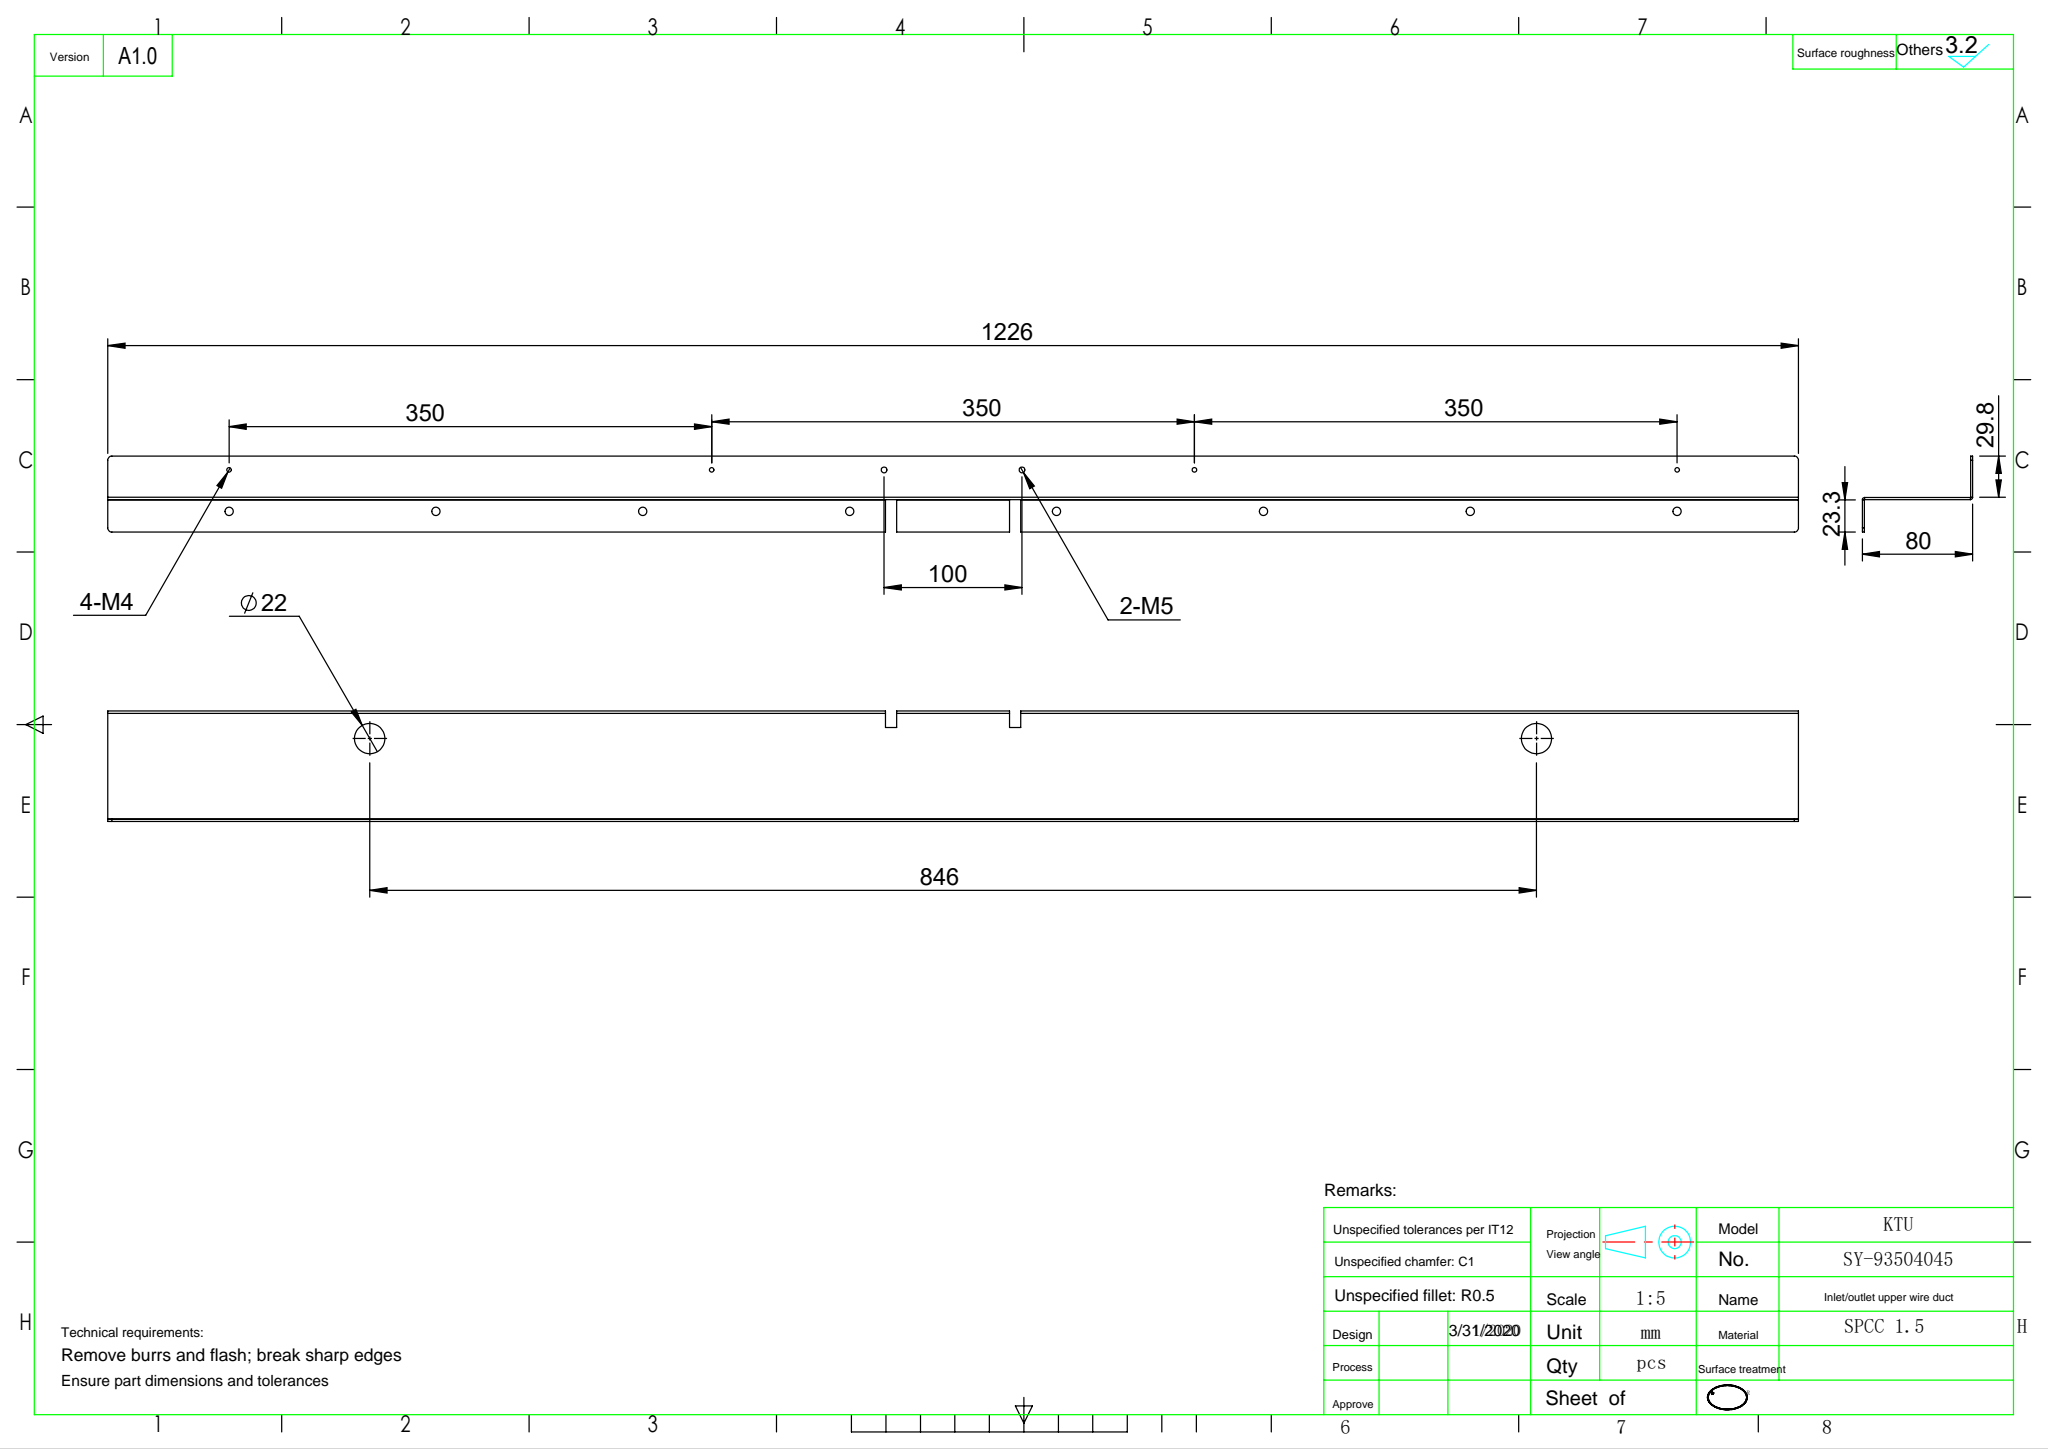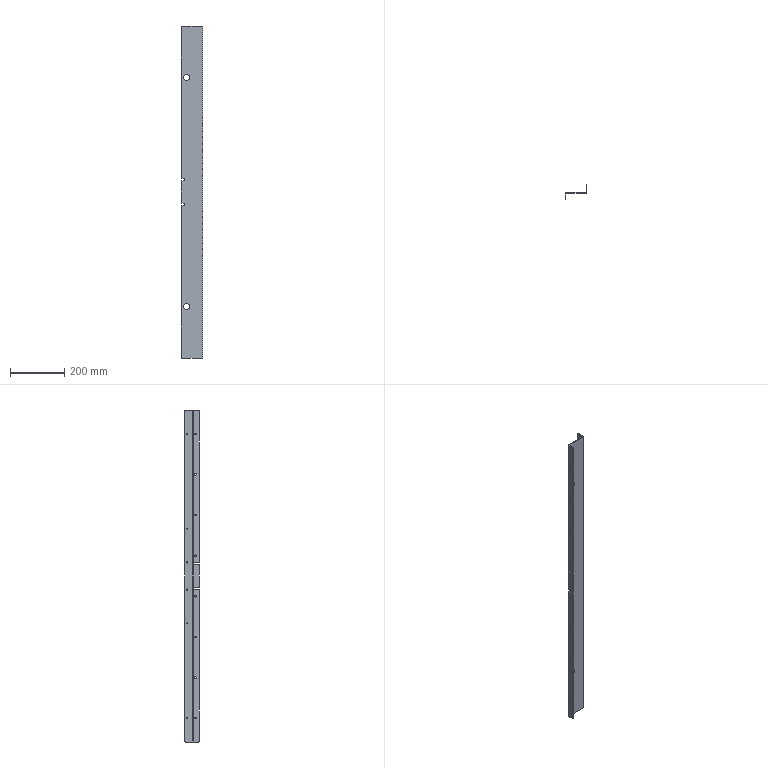Part | SolidWorks | features ICE 3, HoleWzd 2, LPattern 2, Fillet 1, FlatPattern 1, SMBaseFlange 1, SheetMetal 1 | 1 solid | 74 faces | box 80 x 55 x 1226 mm | volume 241580 mm3 | cylinder 44 | plane 30 | commonest cylinder face diameters 6 x20 3.3 x8 0.4 x4 3.4 x4 4.2 x4 22 x4